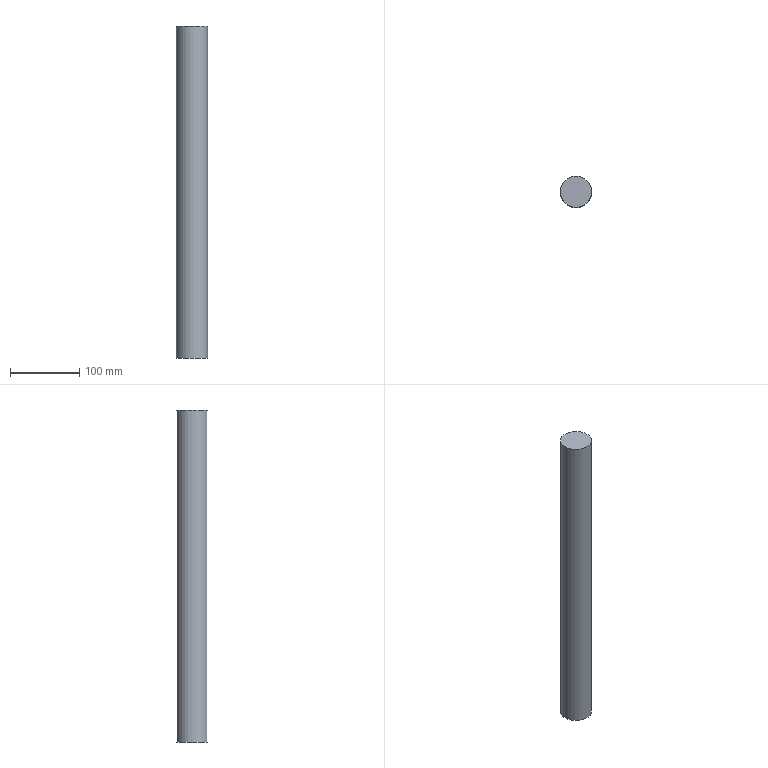Part | NX | features 底座(默认<按焊接>) 2 | 1 solid | 3 faces | box 44.892 x 44.892 x 480 mm | volume 759747 mm3 | plane 2 | cylinder 1 | commonest cylinder face diameters 44.892 x1
STEP:
#1=CARTESIAN_POINT('',(-186.683,240.162,-892.));
#2=VERTEX_POINT('',#1);
#3=CARTESIAN_POINT('',(-209.129,240.162,-892.));
#4=DIRECTION('',(0.,0.,1.));
#5=DIRECTION('',(1.,0.,0.));
#6=AXIS2_PLACEMENT_3D('',#3,#4,#5);
#7=CIRCLE('',#6,22.446);
#8=EDGE_CURVE('',#2,#2,#7,.T.);
#9=ORIENTED_EDGE('',*,*,#8,.T.);
#10=EDGE_LOOP('',(#9));
#11=FACE_BOUND('',#10,.T.);
#12=CARTESIAN_POINT('',(-186.683,240.162,-412.));
#13=VERTEX_POINT('',#12);
#14=CARTESIAN_POINT('',(-209.129,240.162,-412.));
#15=DIRECTION('',(0.,0.,1.));
#16=DIRECTION('',(1.,0.,0.));
#17=AXIS2_PLACEMENT_3D('',#14,#15,#16);
#18=CIRCLE('',#17,22.446);
#19=EDGE_CURVE('',#13,#13,#18,.T.);
#20=ORIENTED_EDGE('',*,*,#19,.F.);
#21=EDGE_LOOP('',(#20));
#22=FACE_BOUND('',#21,.T.);
#23=CARTESIAN_POINT('',(-209.129,240.162,-892.));
#24=DIRECTION('',(0.,0.,1.));
#25=DIRECTION('',(-1.,0.,0.));
#26=AXIS2_PLACEMENT_3D('',#23,#24,#25);
#27=CYLINDRICAL_SURFACE('',#26,22.446);
#28=ADVANCED_FACE('',(#11,#22),#27,.T.);
#29=ORIENTED_EDGE('',*,*,#8,.F.);
#30=EDGE_LOOP('',(#29));
#31=FACE_BOUND('',#30,.T.);
#32=CARTESIAN_POINT('',(1250.85,-2373.536,-892.));
#33=DIRECTION('',(0.,0.,-1.));
#34=DIRECTION('',(1.,0.,0.));
#35=AXIS2_PLACEMENT_3D('',#32,#33,#34);
#36=PLANE('',#35);
#37=ADVANCED_FACE('',(#31),#36,.T.);
#38=ORIENTED_EDGE('',*,*,#19,.T.);
#39=EDGE_LOOP('',(#38));
#40=FACE_BOUND('',#39,.T.);
#41=CARTESIAN_POINT('',(1250.85,-2373.536,-412.));
#42=DIRECTION('',(0.,0.,-1.));
#43=DIRECTION('',(1.,0.,0.));
#44=AXIS2_PLACEMENT_3D('',#41,#42,#43);
#45=PLANE('',#44);
#46=ADVANCED_FACE('',(#40),#45,.F.);
#47=CLOSED_SHELL('',(#28,#37,#46));
#48=MANIFOLD_SOLID_BREP('',#47);
#49=(LENGTH_UNIT()NAMED_UNIT(*)SI_UNIT(.MILLI.,.METRE.));
#50=UNCERTAINTY_MEASURE_WITH_UNIT(LENGTH_MEASURE(0.00001),#49,'','');
#51=(NAMED_UNIT(*)PLANE_ANGLE_UNIT()SI_UNIT($,.RADIAN.));
#52=(NAMED_UNIT(*)SI_UNIT($,.STERADIAN.)SOLID_ANGLE_UNIT());
#53=(GEOMETRIC_REPRESENTATION_CONTEXT(3)GLOBAL_UNCERTAINTY_ASSIGNED_CONTEXT((#50))GLOBAL_UNIT_ASSIGNED_CONTEXT((#49,#51,#52))REPRESENTATION_CONTEXT('',''));
#54=ADVANCED_BREP_SHAPE_REPRESENTATION('',(#48),#53);